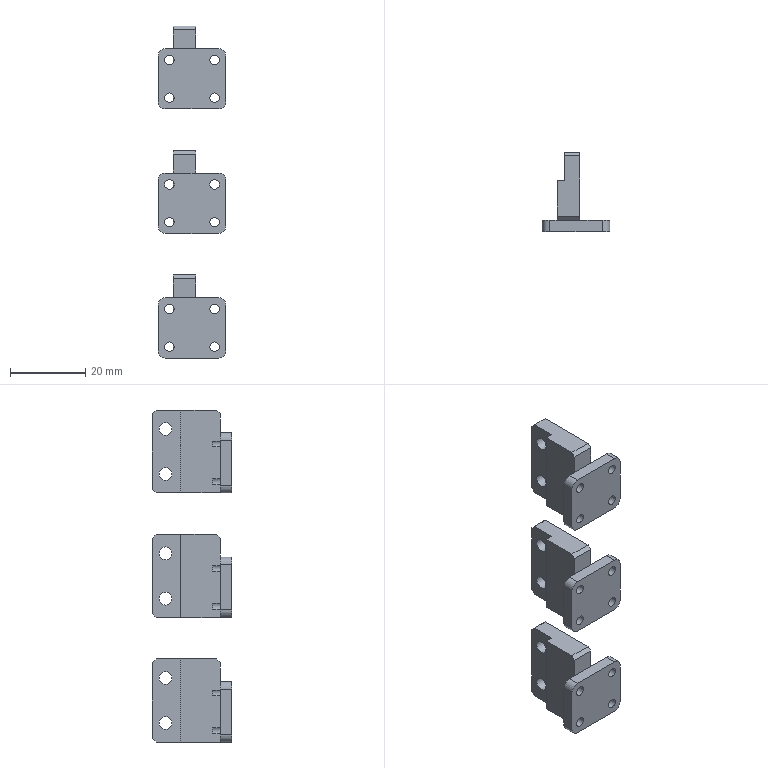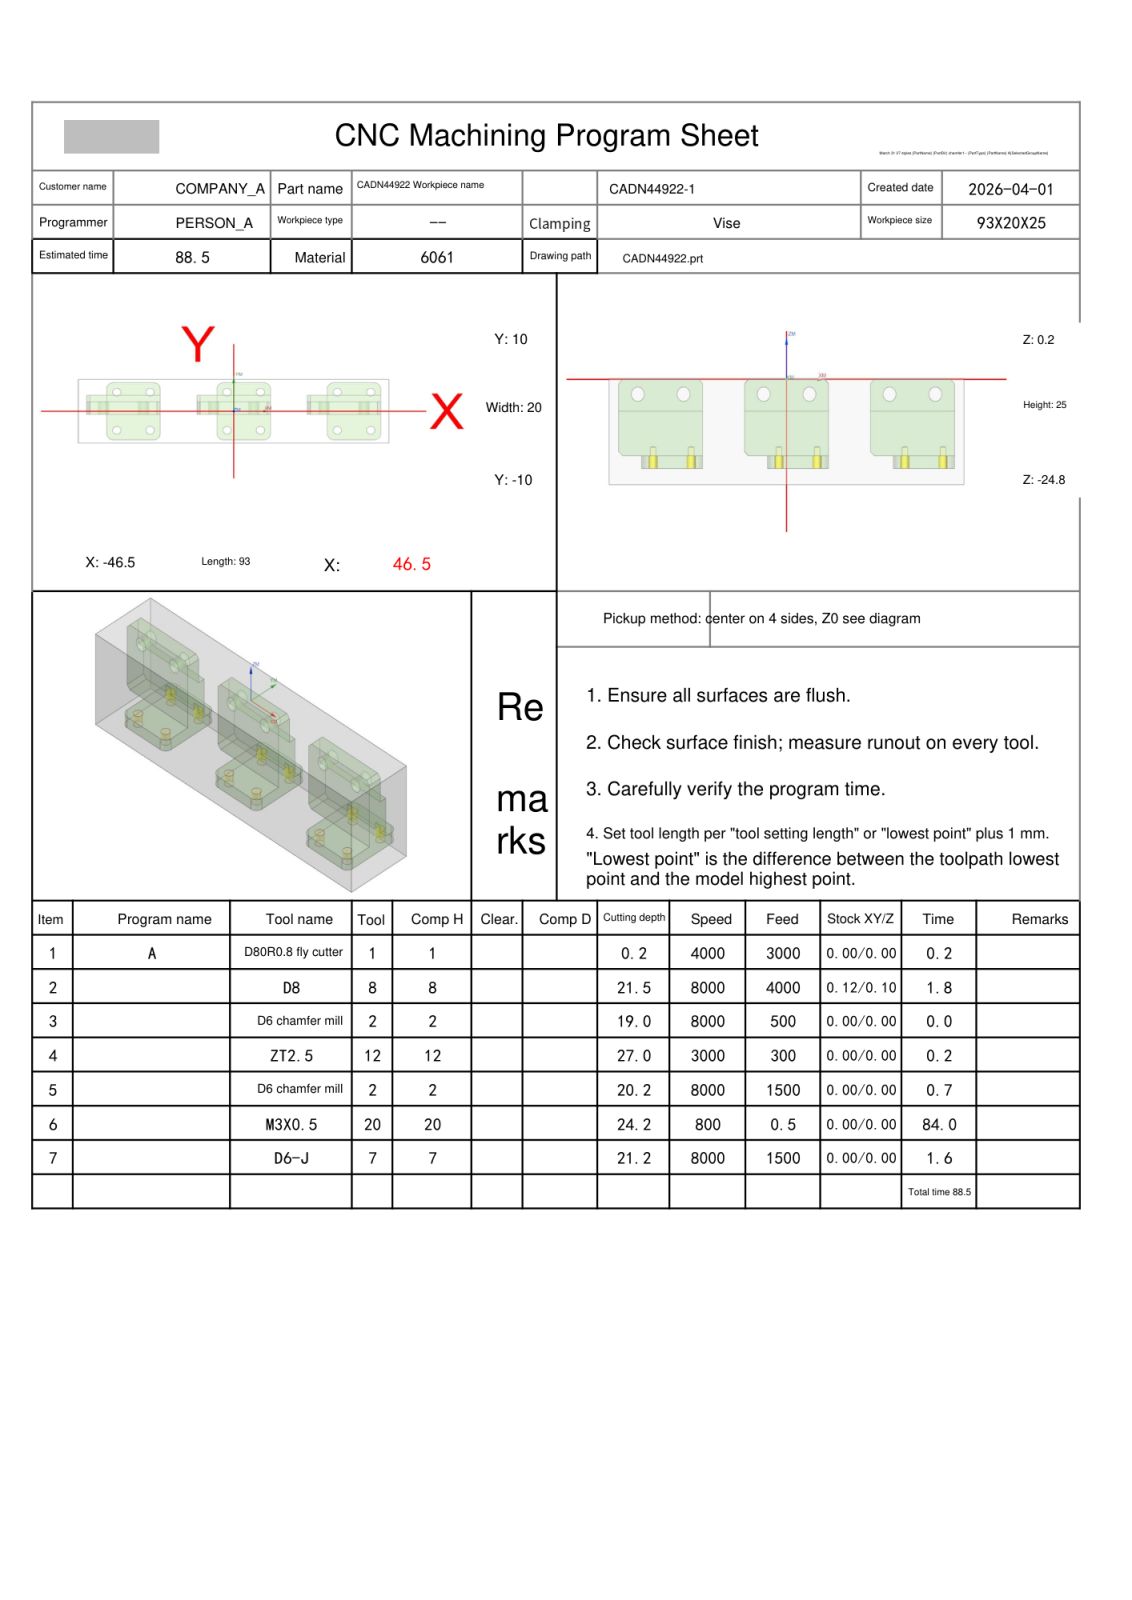NC program | NX | posted by the shop | part box 18 x 21 x 88 mm
Lines 1 to 41 of 4142:
%
O0001
(Machine time: 161.89 MIN)
(===Total Tool:6===)
(T1=D80R0.8 fly cutter D=80.  R=0.8  D-  H01 Z=0.    )
(T8=D8      D=8.   R=0.   D-  H08 Z=-21.3 )
(T2=D6 chamfer mill   D=6.   R=0.   D-  H02 Z=-20.  )
(T12=ZT2.5  D=2.5  DR_a=118 D-  H12 Z=-26.75)
(T20=M3X0.5 D=2.5  DR_a=180 D-  H20 Z=-24.  )
(T7=D6-J    D=6.   R=0.   D7  H07 Z=-21.  )
G80 G90 G17 G49 G40
G91 G28 Z0
M01
N1 T01 M06
(D80R0.8 fly cutter  D=80. R=0.8 H=01 ce=0.20 di=0.10)
G00 G90 G54 X-89. Y0.0 M03 S4000
G43 H01 Z20.
M08
Z2.1
G01 Z.1 F3000.
X-84.
X84.
X89.
Z2.1
G00 Z20.
G00 G90 X-89. Y0.0 M03 S4000
Z20.
Z2.
G01 Z0.0 F1000.
X-84.
X84.
X89.
Z2.
G00 Z20.
G91 G28 Z0.0
M05
M09
G91 G28 Z0.0
M01